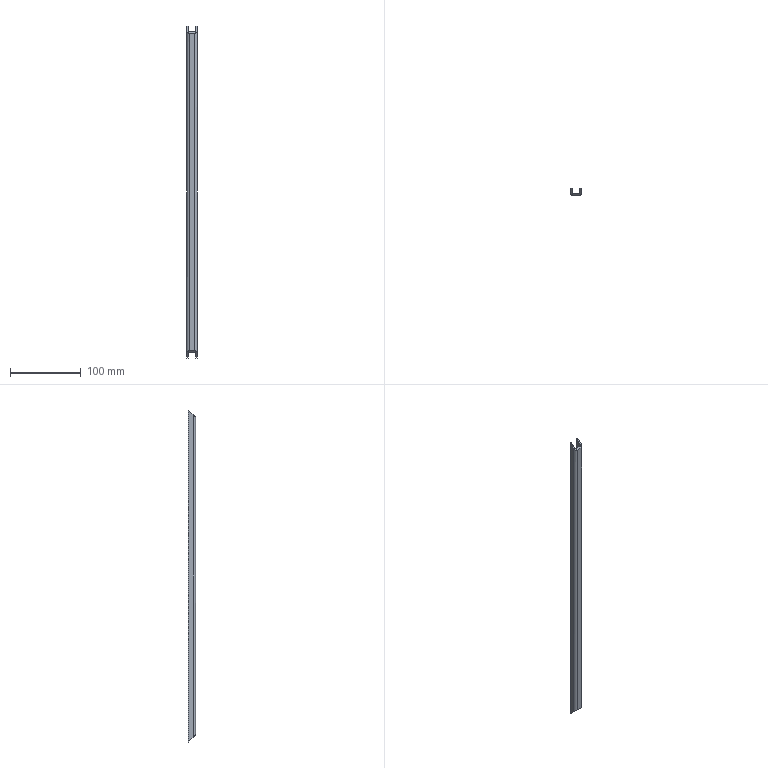Part | STEP file | 1 solid | 14 faces | box 15 x 10 x 470 mm | volume 26409 mm3 | plane 10 | cylinder 4 | commonest cylinder face diameters 3 x2 7 x2
STEP:
#1=CARTESIAN_POINT('',(0.,0.,0.));
#2=DIRECTION('',(0.,0.,1.));
#3=DIRECTION('',(1.,0.,0.));
#4=AXIS2_PLACEMENT_3D('',#1,#2,#3);
#5=CARTESIAN_POINT('',(-5.5,5.,470.));
#6=VERTEX_POINT('',#5);
#7=CARTESIAN_POINT('',(-5.5,5.,0.));
#8=VERTEX_POINT('',#7);
#9=CARTESIAN_POINT('',(-5.5,5.,470.));
#10=DIRECTION('',(0.,0.,-1.));
#11=VECTOR('',#10,1.);
#12=LINE('',#9,#11);
#13=CARTESIAN_POINT('',(-5.5,-5.,470.));
#14=DIRECTION('',(-1.,0.,0.));
#15=DIRECTION('',(0.,0.,1.));
#16=AXIS2_PLACEMENT_3D('',#13,#14,#15);
#17=PLANE('',#16);
#18=CARTESIAN_POINT('',(0.,10.));
#19=DIRECTION('',(-1.,0.));
#20=VECTOR('',#19,1.);
#21=LINE('',#18,#20);
#22=(GEOMETRIC_REPRESENTATION_CONTEXT(2)PARAMETRIC_REPRESENTATION_CONTEXT()REPRESENTATION_CONTEXT('',''));
#23=DEFINITIONAL_REPRESENTATION('',(#21),#22);
#24=PCURVE('',#17,#23);
#25=CARTESIAN_POINT('',(-7.5,5.,470.));
#26=DIRECTION('',(0.,1.,0.));
#27=DIRECTION('',(0.,0.,1.));
#28=AXIS2_PLACEMENT_3D('',#25,#26,#27);
#29=PLANE('',#28);
#30=CARTESIAN_POINT('',(0.,2.));
#31=DIRECTION('',(-1.,0.));
#32=VECTOR('',#31,1.);
#33=LINE('',#30,#32);
#34=(GEOMETRIC_REPRESENTATION_CONTEXT(2)PARAMETRIC_REPRESENTATION_CONTEXT()REPRESENTATION_CONTEXT('',''));
#35=DEFINITIONAL_REPRESENTATION('',(#33),#34);
#36=PCURVE('',#29,#35);
#37=SURFACE_CURVE('',#12,(#24,#36),.PCURVE_S1.);
#38=EDGE_CURVE('',#6,#8,#37,.T.);
#39=ORIENTED_EDGE('',*,*,#38,.F.);
#40=CARTESIAN_POINT('',(-5.5,-1.5,463.5));
#41=VERTEX_POINT('',#40);
#42=CARTESIAN_POINT('',(-5.5,0.,465.));
#43=DIRECTION('',(0.,-0.7071,-0.7071));
#44=VECTOR('',#43,1.);
#45=LINE('',#42,#44);
#46=CARTESIAN_POINT('',(-5.,5.));
#47=DIRECTION('',(-0.7071,-0.7071));
#48=VECTOR('',#47,1.);
#49=LINE('',#46,#48);
#50=(GEOMETRIC_REPRESENTATION_CONTEXT(2)PARAMETRIC_REPRESENTATION_CONTEXT()REPRESENTATION_CONTEXT('',''));
#51=DEFINITIONAL_REPRESENTATION('',(#49),#50);
#52=PCURVE('',#17,#51);
#53=CARTESIAN_POINT('',(-62.5,5.,470.));
#54=DIRECTION('',(0.,0.7071,-0.7071));
#55=DIRECTION('',(0.,0.7071,0.7071));
#56=AXIS2_PLACEMENT_3D('',#53,#54,#55);
#57=PLANE('',#56);
#58=CARTESIAN_POINT('',(-7.071,57.));
#59=DIRECTION('',(-1.,0.));
#60=VECTOR('',#59,1.);
#61=LINE('',#58,#60);
#62=(GEOMETRIC_REPRESENTATION_CONTEXT(2)PARAMETRIC_REPRESENTATION_CONTEXT()REPRESENTATION_CONTEXT('',''));
#63=DEFINITIONAL_REPRESENTATION('',(#61),#62);
#64=PCURVE('',#57,#63);
#65=SURFACE_CURVE('',#45,(#52,#64),.PCURVE_S1.);
#66=EDGE_CURVE('',#6,#41,#65,.T.);
#67=ORIENTED_EDGE('',*,*,#66,.T.);
#68=CARTESIAN_POINT('',(-5.5,-1.5,6.5));
#69=VERTEX_POINT('',#68);
#70=CARTESIAN_POINT('',(-5.5,-1.5,470.));
#71=DIRECTION('',(0.,0.,-1.));
#72=VECTOR('',#71,1.);
#73=LINE('',#70,#72);
#74=CARTESIAN_POINT('',(0.,3.5));
#75=DIRECTION('',(-1.,0.));
#76=VECTOR('',#75,1.);
#77=LINE('',#74,#76);
#78=(GEOMETRIC_REPRESENTATION_CONTEXT(2)PARAMETRIC_REPRESENTATION_CONTEXT()REPRESENTATION_CONTEXT('',''));
#79=DEFINITIONAL_REPRESENTATION('',(#77),#78);
#80=PCURVE('',#17,#79);
#81=CARTESIAN_POINT('',(-4.,-1.5,470.));
#82=DIRECTION('',(0.,0.,-1.));
#83=DIRECTION('',(-1.,0.,0.));
#84=AXIS2_PLACEMENT_3D('',#81,#82,#83);
#85=CYLINDRICAL_SURFACE('',#84,1.5);
#86=CARTESIAN_POINT('',(6.283,0.));
#87=DIRECTION('',(0.,1.));
#88=VECTOR('',#87,1.);
#89=LINE('',#86,#88);
#90=(GEOMETRIC_REPRESENTATION_CONTEXT(2)PARAMETRIC_REPRESENTATION_CONTEXT()REPRESENTATION_CONTEXT('',''));
#91=DEFINITIONAL_REPRESENTATION('',(#89),#90);
#92=PCURVE('',#85,#91);
#93=SURFACE_CURVE('',#73,(#80,#92),.PCURVE_S1.);
#94=EDGE_CURVE('',#41,#69,#93,.T.);
#95=ORIENTED_EDGE('',*,*,#94,.T.);
#96=CARTESIAN_POINT('',(-5.5,-235.,240.));
#97=DIRECTION('',(0.,0.7071,-0.7071));
#98=VECTOR('',#97,1.);
#99=LINE('',#96,#98);
#100=CARTESIAN_POINT('',(-230.,-230.));
#101=DIRECTION('',(-0.7071,0.7071));
#102=VECTOR('',#101,1.);
#103=LINE('',#100,#102);
#104=(GEOMETRIC_REPRESENTATION_CONTEXT(2)PARAMETRIC_REPRESENTATION_CONTEXT()REPRESENTATION_CONTEXT('',''));
#105=DEFINITIONAL_REPRESENTATION('',(#103),#104);
#106=PCURVE('',#17,#105);
#107=CARTESIAN_POINT('',(-62.5,5.,0.));
#108=DIRECTION('',(0.,0.7071,0.7071));
#109=DIRECTION('',(0.,-0.7071,0.7071));
#110=AXIS2_PLACEMENT_3D('',#107,#108,#109);
#111=PLANE('',#110);
#112=CARTESIAN_POINT('',(339.411,57.));
#113=DIRECTION('',(-1.,0.));
#114=VECTOR('',#113,1.);
#115=LINE('',#112,#114);
#116=(GEOMETRIC_REPRESENTATION_CONTEXT(2)PARAMETRIC_REPRESENTATION_CONTEXT()REPRESENTATION_CONTEXT('',''));
#117=DEFINITIONAL_REPRESENTATION('',(#115),#116);
#118=PCURVE('',#111,#117);
#119=SURFACE_CURVE('',#99,(#106,#118),.PCURVE_S1.);
#120=EDGE_CURVE('',#69,#8,#119,.T.);
#121=ORIENTED_EDGE('',*,*,#120,.T.);
#122=EDGE_LOOP('',(#39,#67,#95,#121));
#123=FACE_BOUND('',#122,.T.);
#124=ADVANCED_FACE('',(#123),#17,.F.);
#125=CARTESIAN_POINT('',(-7.5,5.,0.));
#126=VERTEX_POINT('',#125);
#127=CARTESIAN_POINT('',(-7.5,5.,0.));
#128=DIRECTION('',(1.,0.,0.));
#129=VECTOR('',#128,1.);
#130=LINE('',#127,#129);
#131=CARTESIAN_POINT('',(-470.,0.));
#132=DIRECTION('',(0.,1.));
#133=VECTOR('',#132,1.);
#134=LINE('',#131,#133);
#135=(GEOMETRIC_REPRESENTATION_CONTEXT(2)PARAMETRIC_REPRESENTATION_CONTEXT()REPRESENTATION_CONTEXT('',''));
#136=DEFINITIONAL_REPRESENTATION('',(#134),#135);
#137=PCURVE('',#29,#136);
#138=CARTESIAN_POINT('',(0.,55.));
#139=DIRECTION('',(0.,1.));
#140=VECTOR('',#139,1.);
#141=LINE('',#138,#140);
#142=(GEOMETRIC_REPRESENTATION_CONTEXT(2)PARAMETRIC_REPRESENTATION_CONTEXT()REPRESENTATION_CONTEXT('',''));
#143=DEFINITIONAL_REPRESENTATION('',(#141),#142);
#144=PCURVE('',#111,#143);
#145=SURFACE_CURVE('',#130,(#137,#144),.PCURVE_S1.);
#146=EDGE_CURVE('',#126,#8,#145,.T.);
#147=ORIENTED_EDGE('',*,*,#146,.F.);
#148=CARTESIAN_POINT('',(-7.5,5.,470.));
#149=VERTEX_POINT('',#148);
#150=CARTESIAN_POINT('',(-7.5,5.,470.));
#151=DIRECTION('',(0.,0.,-1.));
#152=VECTOR('',#151,1.);
#153=LINE('',#150,#152);
#154=CARTESIAN_POINT('',(0.,0.));
#155=DIRECTION('',(-1.,0.));
#156=VECTOR('',#155,1.);
#157=LINE('',#154,#156);
#158=(GEOMETRIC_REPRESENTATION_CONTEXT(2)PARAMETRIC_REPRESENTATION_CONTEXT()REPRESENTATION_CONTEXT('',''));
#159=DEFINITIONAL_REPRESENTATION('',(#157),#158);
#160=PCURVE('',#29,#159);
#161=CARTESIAN_POINT('',(-7.5,-5.,470.));
#162=DIRECTION('',(-1.,0.,0.));
#163=DIRECTION('',(0.,0.,1.));
#164=AXIS2_PLACEMENT_3D('',#161,#162,#163);
#165=PLANE('',#164);
#166=CARTESIAN_POINT('',(0.,10.));
#167=DIRECTION('',(-1.,0.));
#168=VECTOR('',#167,1.);
#169=LINE('',#166,#168);
#170=(GEOMETRIC_REPRESENTATION_CONTEXT(2)PARAMETRIC_REPRESENTATION_CONTEXT()REPRESENTATION_CONTEXT('',''));
#171=DEFINITIONAL_REPRESENTATION('',(#169),#170);
#172=PCURVE('',#165,#171);
#173=SURFACE_CURVE('',#153,(#160,#172),.PCURVE_S1.);
#174=EDGE_CURVE('',#149,#126,#173,.T.);
#175=ORIENTED_EDGE('',*,*,#174,.F.);
#176=CARTESIAN_POINT('',(-7.5,5.,470.));
#177=DIRECTION('',(1.,0.,0.));
#178=VECTOR('',#177,1.);
#179=LINE('',#176,#178);
#180=CARTESIAN_POINT('',(0.,0.));
#181=DIRECTION('',(0.,1.));
#182=VECTOR('',#181,1.);
#183=LINE('',#180,#182);
#184=(GEOMETRIC_REPRESENTATION_CONTEXT(2)PARAMETRIC_REPRESENTATION_CONTEXT()REPRESENTATION_CONTEXT('',''));
#185=DEFINITIONAL_REPRESENTATION('',(#183),#184);
#186=PCURVE('',#29,#185);
#187=CARTESIAN_POINT('',(0.,55.));
#188=DIRECTION('',(0.,1.));
#189=VECTOR('',#188,1.);
#190=LINE('',#187,#189);
#191=(GEOMETRIC_REPRESENTATION_CONTEXT(2)PARAMETRIC_REPRESENTATION_CONTEXT()REPRESENTATION_CONTEXT('',''));
#192=DEFINITIONAL_REPRESENTATION('',(#190),#191);
#193=PCURVE('',#57,#192);
#194=SURFACE_CURVE('',#179,(#186,#193),.PCURVE_S1.);
#195=EDGE_CURVE('',#149,#6,#194,.T.);
#196=ORIENTED_EDGE('',*,*,#195,.T.);
#197=ORIENTED_EDGE('',*,*,#38,.T.);
#198=EDGE_LOOP('',(#147,#175,#196,#197));
#199=FACE_BOUND('',#198,.T.);
#200=ADVANCED_FACE('',(#199),#29,.T.);
#201=CARTESIAN_POINT('',(-7.5,-1.5,463.5));
#202=VERTEX_POINT('',#201);
#203=CARTESIAN_POINT('',(-7.5,0.,465.));
#204=DIRECTION('',(0.,-0.7071,-0.7071));
#205=VECTOR('',#204,1.);
#206=LINE('',#203,#205);
#207=CARTESIAN_POINT('',(-5.,5.));
#208=DIRECTION('',(-0.7071,-0.7071));
#209=VECTOR('',#208,1.);
#210=LINE('',#207,#209);
#211=(GEOMETRIC_REPRESENTATION_CONTEXT(2)PARAMETRIC_REPRESENTATION_CONTEXT()REPRESENTATION_CONTEXT('',''));
#212=DEFINITIONAL_REPRESENTATION('',(#210),#211);
#213=PCURVE('',#165,#212);
#214=CARTESIAN_POINT('',(-7.071,55.));
#215=DIRECTION('',(-1.,0.));
#216=VECTOR('',#215,1.);
#217=LINE('',#214,#216);
#218=(GEOMETRIC_REPRESENTATION_CONTEXT(2)PARAMETRIC_REPRESENTATION_CONTEXT()REPRESENTATION_CONTEXT('',''));
#219=DEFINITIONAL_REPRESENTATION('',(#217),#218);
#220=PCURVE('',#57,#219);
#221=SURFACE_CURVE('',#206,(#213,#220),.PCURVE_S1.);
#222=EDGE_CURVE('',#149,#202,#221,.T.);
#223=ORIENTED_EDGE('',*,*,#222,.F.);
#224=ORIENTED_EDGE('',*,*,#174,.T.);
#225=CARTESIAN_POINT('',(-7.5,-1.5,6.5));
#226=VERTEX_POINT('',#225);
#227=CARTESIAN_POINT('',(-7.5,-235.,240.));
#228=DIRECTION('',(0.,0.7071,-0.7071));
#229=VECTOR('',#228,1.);
#230=LINE('',#227,#229);
#231=CARTESIAN_POINT('',(-230.,-230.));
#232=DIRECTION('',(-0.7071,0.7071));
#233=VECTOR('',#232,1.);
#234=LINE('',#231,#233);
#235=(GEOMETRIC_REPRESENTATION_CONTEXT(2)PARAMETRIC_REPRESENTATION_CONTEXT()REPRESENTATION_CONTEXT('',''));
#236=DEFINITIONAL_REPRESENTATION('',(#234),#235);
#237=PCURVE('',#165,#236);
#238=CARTESIAN_POINT('',(339.411,55.));
#239=DIRECTION('',(-1.,0.));
#240=VECTOR('',#239,1.);
#241=LINE('',#238,#240);
#242=(GEOMETRIC_REPRESENTATION_CONTEXT(2)PARAMETRIC_REPRESENTATION_CONTEXT()REPRESENTATION_CONTEXT('',''));
#243=DEFINITIONAL_REPRESENTATION('',(#241),#242);
#244=PCURVE('',#111,#243);
#245=SURFACE_CURVE('',#230,(#237,#244),.PCURVE_S1.);
#246=EDGE_CURVE('',#226,#126,#245,.T.);
#247=ORIENTED_EDGE('',*,*,#246,.F.);
#248=CARTESIAN_POINT('',(-7.5,-1.5,470.));
#249=DIRECTION('',(0.,0.,-1.));
#250=VECTOR('',#249,1.);
#251=LINE('',#248,#250);
#252=CARTESIAN_POINT('',(0.,3.5));
#253=DIRECTION('',(-1.,0.));
#254=VECTOR('',#253,1.);
#255=LINE('',#252,#254);
#256=(GEOMETRIC_REPRESENTATION_CONTEXT(2)PARAMETRIC_REPRESENTATION_CONTEXT()REPRESENTATION_CONTEXT('',''));
#257=DEFINITIONAL_REPRESENTATION('',(#255),#256);
#258=PCURVE('',#165,#257);
#259=CARTESIAN_POINT('',(-4.,-1.5,470.));
#260=DIRECTION('',(0.,0.,-1.));
#261=DIRECTION('',(-1.,0.,0.));
#262=AXIS2_PLACEMENT_3D('',#259,#260,#261);
#263=CYLINDRICAL_SURFACE('',#262,3.5);
#264=CARTESIAN_POINT('',(6.283,0.));
#265=DIRECTION('',(0.,1.));
#266=VECTOR('',#265,1.);
#267=LINE('',#264,#266);
#268=(GEOMETRIC_REPRESENTATION_CONTEXT(2)PARAMETRIC_REPRESENTATION_CONTEXT()REPRESENTATION_CONTEXT('',''));
#269=DEFINITIONAL_REPRESENTATION('',(#267),#268);
#270=PCURVE('',#263,#269);
#271=SURFACE_CURVE('',#251,(#258,#270),.PCURVE_S1.);
#272=EDGE_CURVE('',#202,#226,#271,.T.);
#273=ORIENTED_EDGE('',*,*,#272,.F.);
#274=EDGE_LOOP('',(#223,#224,#247,#273));
#275=FACE_BOUND('',#274,.T.);
#276=ADVANCED_FACE('',(#275),#165,.T.);
#277=CARTESIAN_POINT('',(-4.,-5.,460.));
#278=VERTEX_POINT('',#277);
#279=CARTESIAN_POINT('',(-7.5,-1.5,463.5));
#280=CARTESIAN_POINT('',(-7.5,-3.55,461.45));
#281=CARTESIAN_POINT('',(-6.05,-5.,460.));
#282=CARTESIAN_POINT('',(-4.,-5.,460.));
#283=(BOUNDED_CURVE()B_SPLINE_CURVE(3,(#279,#280,#281,#282),.UNSPECIFIED.,.F.,.F.)B_SPLINE_CURVE_WITH_KNOTS((4,4),(4.712,6.283),.PIECEWISE_BEZIER_KNOTS.)CURVE()GEOMETRIC_REPRESENTATION_ITEM()RATIONAL_B_SPLINE_CURVE((1.,0.8047,0.8047,1.))REPRESENTATION_ITEM(''));
#284=CARTESIAN_POINT('',(6.283,6.5));
#285=CARTESIAN_POINT('',(6.262,6.575));
#286=CARTESIAN_POINT('',(6.218,6.727));
#287=CARTESIAN_POINT('',(6.152,6.96));
#288=CARTESIAN_POINT('',(6.083,7.196));
#289=CARTESIAN_POINT('',(6.013,7.433));
#290=CARTESIAN_POINT('',(5.942,7.671));
#291=CARTESIAN_POINT('',(5.87,7.906));
#292=CARTESIAN_POINT('',(5.797,8.137));
#293=CARTESIAN_POINT('',(5.723,8.362));
#294=CARTESIAN_POINT('',(5.648,8.578));
#295=CARTESIAN_POINT('',(5.573,8.784));
#296=CARTESIAN_POINT('',(5.498,8.977));
#297=CARTESIAN_POINT('',(5.422,9.157));
#298=CARTESIAN_POINT('',(5.347,9.32));
#299=CARTESIAN_POINT('',(5.273,9.468));
#300=CARTESIAN_POINT('',(5.199,9.597));
#301=CARTESIAN_POINT('',(5.125,9.709));
#302=CARTESIAN_POINT('',(5.053,9.802));
#303=CARTESIAN_POINT('',(4.982,9.876));
#304=CARTESIAN_POINT('',(4.912,9.933));
#305=CARTESIAN_POINT('',(4.844,9.972));
#306=CARTESIAN_POINT('',(4.777,9.995));
#307=CARTESIAN_POINT('',(4.734,10.));
#308=CARTESIAN_POINT('',(4.712,10.));
#309=B_SPLINE_CURVE_WITH_KNOTS('',3,(#284,#285,#286,#287,#288,#289,#290,#291,#292,#293,#294,#295,#296,#297,#298,#299,#300,#301,#302,#303,#304,#305,#306,#307,#308),.UNSPECIFIED.,.F.,.F.,(4,1,1,1,1,1,1,1,1,1,1,1,1,1,1,1,1,1,1,1,1,1,4),(4.712,4.784,4.855,4.927,4.998,5.069,5.141,5.212,5.284,5.355,5.426,5.498,5.569,5.641,5.712,5.783,5.855,5.926,5.998,6.069,6.14,6.212,6.283),.QUASI_UNIFORM_KNOTS.);
#310=(GEOMETRIC_REPRESENTATION_CONTEXT(2)PARAMETRIC_REPRESENTATION_CONTEXT()REPRESENTATION_CONTEXT('',''));
#311=DEFINITIONAL_REPRESENTATION('',(#309),#310);
#312=PCURVE('',#263,#311);
#313=CARTESIAN_POINT('',(-9.192,55.));
#314=CARTESIAN_POINT('',(-12.092,55.));
#315=CARTESIAN_POINT('',(-14.142,56.45));
#316=CARTESIAN_POINT('',(-14.142,58.5));
#317=(BOUNDED_CURVE()B_SPLINE_CURVE(3,(#313,#314,#315,#316),.UNSPECIFIED.,.F.,.F.)B_SPLINE_CURVE_WITH_KNOTS((4,4),(4.712,6.283),.PIECEWISE_BEZIER_KNOTS.)CURVE()GEOMETRIC_REPRESENTATION_ITEM()RATIONAL_B_SPLINE_CURVE((1.,0.8047,0.8047,1.))REPRESENTATION_ITEM(''));
#318=(GEOMETRIC_REPRESENTATION_CONTEXT(2)PARAMETRIC_REPRESENTATION_CONTEXT()REPRESENTATION_CONTEXT('',''));
#319=DEFINITIONAL_REPRESENTATION('',(#317),#318);
#320=PCURVE('',#57,#319);
#321=SURFACE_CURVE('',#283,(#312,#320),.PCURVE_S1.);
#322=EDGE_CURVE('',#202,#278,#321,.T.);
#323=ORIENTED_EDGE('',*,*,#322,.F.);
#324=ORIENTED_EDGE('',*,*,#272,.T.);
#325=CARTESIAN_POINT('',(-4.,-5.,10.));
#326=VERTEX_POINT('',#325);
#327=CARTESIAN_POINT('',(-4.,-5.,10.));
#328=CARTESIAN_POINT('',(-6.05,-5.,10.));
#329=CARTESIAN_POINT('',(-7.5,-3.55,8.55));
#330=CARTESIAN_POINT('',(-7.5,-1.5,6.5));
#331=(BOUNDED_CURVE()B_SPLINE_CURVE(3,(#327,#328,#329,#330),.UNSPECIFIED.,.F.,.F.)B_SPLINE_CURVE_WITH_KNOTS((4,4),(3.142,4.712),.PIECEWISE_BEZIER_KNOTS.)CURVE()GEOMETRIC_REPRESENTATION_ITEM()RATIONAL_B_SPLINE_CURVE((1.,0.8047,0.8047,1.))REPRESENTATION_ITEM(''));
#332=CARTESIAN_POINT('',(4.712,460.));
#333=CARTESIAN_POINT('',(4.734,460.));
#334=CARTESIAN_POINT('',(4.777,460.005));
#335=CARTESIAN_POINT('',(4.844,460.028));
#336=CARTESIAN_POINT('',(4.912,460.067));
#337=CARTESIAN_POINT('',(4.982,460.124));
#338=CARTESIAN_POINT('',(5.053,460.198));
#339=CARTESIAN_POINT('',(5.125,460.291));
#340=CARTESIAN_POINT('',(5.199,460.403));
#341=CARTESIAN_POINT('',(5.273,460.532));
#342=CARTESIAN_POINT('',(5.347,460.68));
#343=CARTESIAN_POINT('',(5.422,460.843));
#344=CARTESIAN_POINT('',(5.498,461.023));
#345=CARTESIAN_POINT('',(5.573,461.216));
#346=CARTESIAN_POINT('',(5.648,461.422));
#347=CARTESIAN_POINT('',(5.723,461.638));
#348=CARTESIAN_POINT('',(5.797,461.863));
#349=CARTESIAN_POINT('',(5.87,462.094));
#350=CARTESIAN_POINT('',(5.942,462.329));
#351=CARTESIAN_POINT('',(6.013,462.567));
#352=CARTESIAN_POINT('',(6.083,462.804));
#353=CARTESIAN_POINT('',(6.152,463.04));
#354=CARTESIAN_POINT('',(6.218,463.273));
#355=CARTESIAN_POINT('',(6.262,463.425));
#356=CARTESIAN_POINT('',(6.283,463.5));
#357=B_SPLINE_CURVE_WITH_KNOTS('',3,(#332,#333,#334,#335,#336,#337,#338,#339,#340,#341,#342,#343,#344,#345,#346,#347,#348,#349,#350,#351,#352,#353,#354,#355,#356),.UNSPECIFIED.,.F.,.F.,(4,1,1,1,1,1,1,1,1,1,1,1,1,1,1,1,1,1,1,1,1,1,4),(3.142,3.213,3.284,3.356,3.427,3.499,3.57,3.641,3.713,3.784,3.856,3.927,3.998,4.07,4.141,4.213,4.284,4.355,4.427,4.498,4.57,4.641,4.712),.QUASI_UNIFORM_KNOTS.);
#358=(GEOMETRIC_REPRESENTATION_CONTEXT(2)PARAMETRIC_REPRESENTATION_CONTEXT()REPRESENTATION_CONTEXT('',''));
#359=DEFINITIONAL_REPRESENTATION('',(#357),#358);
#360=PCURVE('',#263,#359);
#361=CARTESIAN_POINT('',(14.142,58.5));
#362=CARTESIAN_POINT('',(14.142,56.45));
#363=CARTESIAN_POINT('',(12.092,55.));
#364=CARTESIAN_POINT('',(9.192,55.));
#365=(BOUNDED_CURVE()B_SPLINE_CURVE(3,(#361,#362,#363,#364),.UNSPECIFIED.,.F.,.F.)B_SPLINE_CURVE_WITH_KNOTS((4,4),(3.142,4.712),.PIECEWISE_BEZIER_KNOTS.)CURVE()GEOMETRIC_REPRESENTATION_ITEM()RATIONAL_B_SPLINE_CURVE((1.,0.8047,0.8047,1.))REPRESENTATION_ITEM(''));
#366=(GEOMETRIC_REPRESENTATION_CONTEXT(2)PARAMETRIC_REPRESENTATION_CONTEXT()REPRESENTATION_CONTEXT('',''));
#367=DEFINITIONAL_REPRESENTATION('',(#365),#366);
#368=PCURVE('',#111,#367);
#369=SURFACE_CURVE('',#331,(#360,#368),.PCURVE_S1.);
#370=EDGE_CURVE('',#326,#226,#369,.T.);
#371=ORIENTED_EDGE('',*,*,#370,.F.);
#372=CARTESIAN_POINT('',(-4.,-5.,470.));
#373=DIRECTION('',(0.,0.,-1.));
#374=VECTOR('',#373,1.);
#375=LINE('',#372,#374);
#376=CARTESIAN_POINT('',(4.712,0.));
#377=DIRECTION('',(0.,1.));
#378=VECTOR('',#377,1.);
#379=LINE('',#376,#378);
#380=(GEOMETRIC_REPRESENTATION_CONTEXT(2)PARAMETRIC_REPRESENTATION_CONTEXT()REPRESENTATION_CONTEXT('',''));
#381=DEFINITIONAL_REPRESENTATION('',(#379),#380);
#382=PCURVE('',#263,#381);
#383=CARTESIAN_POINT('',(-7.5,-5.,470.));
#384=DIRECTION('',(0.,-1.,0.));
#385=DIRECTION('',(0.,0.,-1.));
#386=AXIS2_PLACEMENT_3D('',#383,#384,#385);
#387=PLANE('',#386);
#388=CARTESIAN_POINT('',(0.,3.5));
#389=DIRECTION('',(1.,0.));
#390=VECTOR('',#389,1.);
#391=LINE('',#388,#390);
#392=(GEOMETRIC_REPRESENTATION_CONTEXT(2)PARAMETRIC_REPRESENTATION_CONTEXT()REPRESENTATION_CONTEXT('',''));
#393=DEFINITIONAL_REPRESENTATION('',(#391),#392);
#394=PCURVE('',#387,#393);
#395=SURFACE_CURVE('',#375,(#382,#394),.PCURVE_S1.);
#396=EDGE_CURVE('',#278,#326,#395,.T.);
#397=ORIENTED_EDGE('',*,*,#396,.F.);
#398=EDGE_LOOP('',(#323,#324,#371,#397));
#399=FACE_BOUND('',#398,.T.);
#400=ADVANCED_FACE('',(#399),#263,.T.);
#401=CARTESIAN_POINT('',(4.,-5.,460.));
#402=VERTEX_POINT('',#401);
#403=CARTESIAN_POINT('',(-62.5,-5.,460.));
#404=DIRECTION('',(1.,0.,0.));
#405=VECTOR('',#404,1.);
#406=LINE('',#403,#405);
#407=CARTESIAN_POINT('',(10.,-55.));
#408=DIRECTION('',(0.,1.));
#409=VECTOR('',#408,1.);
#410=LINE('',#407,#409);
#411=(GEOMETRIC_REPRESENTATION_CONTEXT(2)PARAMETRIC_REPRESENTATION_CONTEXT()REPRESENTATION_CONTEXT('',''));
#412=DEFINITIONAL_REPRESENTATION('',(#410),#411);
#413=PCURVE('',#387,#412);
#414=CARTESIAN_POINT('',(-14.142,0.));
#415=DIRECTION('',(0.,1.));
#416=VECTOR('',#415,1.);
#417=LINE('',#414,#416);
#418=(GEOMETRIC_REPRESENTATION_CONTEXT(2)PARAMETRIC_REPRESENTATION_CONTEXT()REPRESENTATION_CONTEXT('',''));
#419=DEFINITIONAL_REPRESENTATION('',(#417),#418);
#420=PCURVE('',#57,#419);
#421=SURFACE_CURVE('',#406,(#413,#420),.PCURVE_S1.);
#422=EDGE_CURVE('',#278,#402,#421,.T.);
#423=ORIENTED_EDGE('',*,*,#422,.F.);
#424=ORIENTED_EDGE('',*,*,#396,.T.);
#425=CARTESIAN_POINT('',(4.,-5.,10.));
#426=VERTEX_POINT('',#425);
#427=CARTESIAN_POINT('',(-62.5,-5.,10.));
#428=DIRECTION('',(1.,0.,0.));
#429=VECTOR('',#428,1.);
#430=LINE('',#427,#429);
#431=CARTESIAN_POINT('',(460.,-55.));
#432=DIRECTION('',(0.,1.));
#433=VECTOR('',#432,1.);
#434=LINE('',#431,#433);
#435=(GEOMETRIC_REPRESENTATION_CONTEXT(2)PARAMETRIC_REPRESENTATION_CONTEXT()REPRESENTATION_CONTEXT('',''));
#436=DEFINITIONAL_REPRESENTATION('',(#434),#435);
#437=PCURVE('',#387,#436);
#438=CARTESIAN_POINT('',(14.142,0.));
#439=DIRECTION('',(0.,1.));
#440=VECTOR('',#439,1.);
#441=LINE('',#438,#440);
#442=(GEOMETRIC_REPRESENTATION_CONTEXT(2)PARAMETRIC_REPRESENTATION_CONTEXT()REPRESENTATION_CONTEXT('',''));
#443=DEFINITIONAL_REPRESENTATION('',(#441),#442);
#444=PCURVE('',#111,#443);
#445=SURFACE_CURVE('',#430,(#437,#444),.PCURVE_S1.);
#446=EDGE_CURVE('',#326,#426,#445,.T.);
#447=ORIENTED_EDGE('',*,*,#446,.T.);
#448=CARTESIAN_POINT('',(4.,-5.,470.));
#449=DIRECTION('',(0.,0.,-1.));
#450=VECTOR('',#449,1.);
#451=LINE('',#448,#450);
#452=CARTESIAN_POINT('',(0.,11.5));
#453=DIRECTION('',(1.,0.));
#454=VECTOR('',#453,1.);
#455=LINE('',#452,#454);
#456=(GEOMETRIC_REPRESENTATION_CONTEXT(2)PARAMETRIC_REPRESENTATION_CONTEXT()REPRESENTATION_CONTEXT('',''));
#457=DEFINITIONAL_REPRESENTATION('',(#455),#456);
#458=PCURVE('',#387,#457);
#459=CARTESIAN_POINT('',(4.,-1.5,470.));
#460=DIRECTION('',(0.,0.,-1.));
#461=DIRECTION('',(-1.,0.,0.));
#462=AXIS2_PLACEMENT_3D('',#459,#460,#461);
#463=CYLINDRICAL_SURFACE('',#462,3.5);
#464=CARTESIAN_POINT('',(4.712,0.));
#465=DIRECTION('',(0.,1.));
#466=VECTOR('',#465,1.);
#467=LINE('',#464,#466);
#468=(GEOMETRIC_REPRESENTATION_CONTEXT(2)PARAMETRIC_REPRESENTATION_CONTEXT()REPRESENTATION_CONTEXT('',''));
#469=DEFINITIONAL_REPRESENTATION('',(#467),#468);
#470=PCURVE('',#463,#469);
#471=SURFACE_CURVE('',#451,(#458,#470),.PCURVE_S1.);
#472=EDGE_CURVE('',#402,#426,#471,.T.);
#473=ORIENTED_EDGE('',*,*,#472,.F.);
#474=EDGE_LOOP('',(#423,#424,#447,#473));
#475=FACE_BOUND('',#474,.T.);
#476=ADVANCED_FACE('',(#475),#387,.T.);
#477=CARTESIAN_POINT('',(7.5,-1.5,463.5));
#478=VERTEX_POINT('',#477);
#479=CARTESIAN_POINT('',(4.,-5.,460.));
#480=CARTESIAN_POINT('',(6.05,-5.,460.));
#481=CARTESIAN_POINT('',(7.5,-3.55,461.45));
#482=CARTESIAN_POINT('',(7.5,-1.5,463.5));
#483=(BOUNDED_CURVE()B_SPLINE_CURVE(3,(#479,#480,#481,#482),.UNSPECIFIED.,.F.,.F.)B_SPLINE_CURVE_WITH_KNOTS((4,4),(0.,1.571),.PIECEWISE_BEZIER_KNOTS.)CURVE()GEOMETRIC_REPRESENTATION_ITEM()RATIONAL_B_SPLINE_CURVE((1.,0.8047,0.8047,1.))REPRESENTATION_ITEM(''));
#484=CARTESIAN_POINT('',(4.712,10.));
#485=CARTESIAN_POINT('',(4.691,10.));
#486=CARTESIAN_POINT('',(4.648,9.995));
#487=CARTESIAN_POINT('',(4.581,9.972));
#488=CARTESIAN_POINT('',(4.512,9.933));
#489=CARTESIAN_POINT('',(4.443,9.876));
#490=CARTESIAN_POINT('',(4.372,9.802));
#491=CARTESIAN_POINT('',(4.299,9.709));
#492=CARTESIAN_POINT('',(4.226,9.597));
#493=CARTESIAN_POINT('',(4.152,9.468));
#494=CARTESIAN_POINT('',(4.077,9.32));
#495=CARTESIAN_POINT('',(4.002,9.157));
#496=CARTESIAN_POINT('',(3.927,8.977));
#497=CARTESIAN_POINT('',(3.852,8.784));
#498=CARTESIAN_POINT('',(3.777,8.578));
#499=CARTESIAN_POINT('',(3.702,8.362));
#500=CARTESIAN_POINT('',(3.628,8.137));
#501=CARTESIAN_POINT('',(3.555,7.906));
#502=CARTESIAN_POINT('',(3.482,7.671));
#503=CARTESIAN_POINT('',(3.411,7.433));
#504=CARTESIAN_POINT('',(3.342,7.196));
#505=CARTESIAN_POINT('',(3.273,6.96));
#506=CARTESIAN_POINT('',(3.206,6.727));
#507=CARTESIAN_POINT('',(3.163,6.575));
#508=CARTESIAN_POINT('',(3.142,6.5));
#509=B_SPLINE_CURVE_WITH_KNOTS('',3,(#484,#485,#486,#487,#488,#489,#490,#491,#492,#493,#494,#495,#496,#497,#498,#499,#500,#501,#502,#503,#504,#505,#506,#507,#508),.UNSPECIFIED.,.F.,.F.,(4,1,1,1,1,1,1,1,1,1,1,1,1,1,1,1,1,1,1,1,1,1,4),(0.,0.0714,0.1428,0.2142,0.2856,0.357,0.4284,0.4998,0.5712,0.6426,0.714,0.7854,0.8568,0.9282,0.9996,1.071,1.142,1.214,1.285,1.357,1.428,1.499,1.571),.QUASI_UNIFORM_KNOTS.);
#510=(GEOMETRIC_REPRESENTATION_CONTEXT(2)PARAMETRIC_REPRESENTATION_CONTEXT()REPRESENTATION_CONTEXT('',''));
#511=DEFINITIONAL_REPRESENTATION('',(#509),#510);
#512=PCURVE('',#463,#511);
#513=CARTESIAN_POINT('',(-14.142,66.5));
#514=CARTESIAN_POINT('',(-14.142,68.55));
#515=CARTESIAN_POINT('',(-12.092,70.));
#516=CARTESIAN_POINT('',(-9.192,70.));
#517=(BOUNDED_CURVE()B_SPLINE_CURVE(3,(#513,#514,#515,#516),.UNSPECIFIED.,.F.,.F.)B_SPLINE_CURVE_WITH_KNOTS((4,4),(0.,1.571),.PIECEWISE_BEZIER_KNOTS.)CURVE()GEOMETRIC_REPRESENTATION_ITEM()RATIONAL_B_SPLINE_CURVE((1.,0.8047,0.8047,1.))REPRESENTATION_ITEM(''));
#518=(GEOMETRIC_REPRESENTATION_CONTEXT(2)PARAMETRIC_REPRESENTATION_CONTEXT()REPRESENTATION_CONTEXT('',''));
#519=DEFINITIONAL_REPRESENTATION('',(#517),#518);
#520=PCURVE('',#57,#519);
#521=SURFACE_CURVE('',#483,(#512,#520),.PCURVE_S1.);
#522=EDGE_CURVE('',#402,#478,#521,.T.);
#523=ORIENTED_EDGE('',*,*,#522,.F.);
#524=ORIENTED_EDGE('',*,*,#472,.T.);
#525=CARTESIAN_POINT('',(7.5,-1.5,6.5));
#526=VERTEX_POINT('',#525);
#527=CARTESIAN_POINT('',(7.5,-1.5,6.5));
#528=CARTESIAN_POINT('',(7.5,-3.55,8.55));
#529=CARTESIAN_POINT('',(6.05,-5.,10.));
#530=CARTESIAN_POINT('',(4.,-5.,10.));
#531=(BOUNDED_CURVE()B_SPLINE_CURVE(3,(#527,#528,#529,#530),.UNSPECIFIED.,.F.,.F.)B_SPLINE_CURVE_WITH_KNOTS((4,4),(1.571,3.142),.PIECEWISE_BEZIER_KNOTS.)CURVE()GEOMETRIC_REPRESENTATION_ITEM()RATIONAL_B_SPLINE_CURVE((1.,0.8047,0.8047,1.))REPRESENTATION_ITEM(''));
#532=CARTESIAN_POINT('',(3.142,463.5));
#533=CARTESIAN_POINT('',(3.163,463.425));
#534=CARTESIAN_POINT('',(3.206,463.273));
#535=CARTESIAN_POINT('',(3.273,463.04));
#536=CARTESIAN_POINT('',(3.342,462.804));
#537=CARTESIAN_POINT('',(3.411,462.567));
#538=CARTESIAN_POINT('',(3.482,462.329));
#539=CARTESIAN_POINT('',(3.555,462.094));
#540=CARTESIAN_POINT('',(3.628,461.863));
#541=CARTESIAN_POINT('',(3.702,461.638));
#542=CARTESIAN_POINT('',(3.777,461.422));
#543=CARTESIAN_POINT('',(3.852,461.216));
#544=CARTESIAN_POINT('',(3.927,461.023));
#545=CARTESIAN_POINT('',(4.002,460.843));
#546=CARTESIAN_POINT('',(4.077,460.68));
#547=CARTESIAN_POINT('',(4.152,460.532));
#548=CARTESIAN_POINT('',(4.226,460.403));
#549=CARTESIAN_POINT('',(4.299,460.291));
#550=CARTESIAN_POINT('',(4.372,460.198));
#551=CARTESIAN_POINT('',(4.443,460.124));
#552=CARTESIAN_POINT('',(4.512,460.067));
#553=CARTESIAN_POINT('',(4.581,460.028));
#554=CARTESIAN_POINT('',(4.648,460.005));
#555=CARTESIAN_POINT('',(4.691,460.));
#556=CARTESIAN_POINT('',(4.712,460.));
#557=B_SPLINE_CURVE_WITH_KNOTS('',3,(#532,#533,#534,#535,#536,#537,#538,#539,#540,#541,#542,#543,#544,#545,#546,#547,#548,#549,#550,#551,#552,#553,#554,#555,#556),.UNSPECIFIED.,.F.,.F.,(4,1,1,1,1,1,1,1,1,1,1,1,1,1,1,1,1,1,1,1,1,1,4),(1.571,1.642,1.714,1.785,1.856,1.928,1.999,2.071,2.142,2.213,2.285,2.356,2.428,2.499,2.57,2.642,2.713,2.785,2.856,2.927,2.999,3.07,3.142),.QUASI_UNIFORM_KNOTS.);
#558=(GEOMETRIC_REPRESENTATION_CONTEXT(2)PARAMETRIC_REPRESENTATION_CONTEXT()REPRESENTATION_CONTEXT('',''));
#559=DEFINITIONAL_REPRESENTATION('',(#557),#558);
#560=PCURVE('',#463,#559);
#561=CARTESIAN_POINT('',(9.192,70.));
#562=CARTESIAN_POINT('',(12.092,70.));
#563=CARTESIAN_POINT('',(14.142,68.55));
#564=CARTESIAN_POINT('',(14.142,66.5));
#565=(BOUNDED_CURVE()B_SPLINE_CURVE(3,(#561,#562,#563,#564),.UNSPECIFIED.,.F.,.F.)B_SPLINE_CURVE_WITH_KNOTS((4,4),(1.571,3.142),.PIECEWISE_BEZIER_KNOTS.)CURVE()GEOMETRIC_REPRESENTATION_ITEM()RATIONAL_B_SPLINE_CURVE((1.,0.8047,0.8047,1.))REPRESENTATION_ITEM(''));
#566=(GEOMETRIC_REPRESENTATION_CONTEXT(2)PARAMETRIC_REPRESENTATION_CONTEXT()REPRESENTATION_CONTEXT('',''));
#567=DEFINITIONAL_REPRESENTATION('',(#565),#566);
#568=PCURVE('',#111,#567);
#569=SURFACE_CURVE('',#531,(#560,#568),.PCURVE_S1.);
#570=EDGE_CURVE('',#526,#426,#569,.T.);
#571=ORIENTED_EDGE('',*,*,#570,.F.);
#572=CARTESIAN_POINT('',(7.5,-1.5,470.));
#573=DIRECTION('',(0.,0.,-1.));
#574=VECTOR('',#573,1.);
#575=LINE('',#572,#574);
#576=CARTESIAN_POINT('',(3.142,0.));
#577=DIRECTION('',(0.,1.));
#578=VECTOR('',#577,1.);
#579=LINE('',#576,#578);
#580=(GEOMETRIC_REPRESENTATION_CONTEXT(2)PARAMETRIC_REPRESENTATION_CONTEXT()REPRESENTATION_CONTEXT('',''));
#581=DEFINITIONAL_REPRESENTATION('',(#579),#580);
#582=PCURVE('',#463,#581);
#583=CARTESIAN_POINT('',(7.5,-5.,470.));
#584=DIRECTION('',(1.,0.,0.));
#585=DIRECTION('',(0.,0.,-1.));
#586=AXIS2_PLACEMENT_3D('',#583,#584,#585);
#587=PLANE('',#586);
#588=CARTESIAN_POINT('',(0.,3.5));
#589=DIRECTION('',(1.,0.));
#590=VECTOR('',#589,1.);
#591=LINE('',#588,#590);
#592=(GEOMETRIC_REPRESENTATION_CONTEXT(2)PARAMETRIC_REPRESENTATION_CONTEXT()REPRESENTATION_CONTEXT('',''));
#593=DEFINITIONAL_REPRESENTATION('',(#591),#592);
#594=PCURVE('',#587,#593);
#595=SURFACE_CURVE('',#575,(#582,#594),.PCURVE_S1.);
#596=EDGE_CURVE('',#478,#526,#595,.T.);
#597=ORIENTED_EDGE('',*,*,#596,.F.);
#598=EDGE_LOOP('',(#523,#524,#571,#597));
#599=FACE_BOUND('',#598,.T.);
#600=ADVANCED_FACE('',(#599),#463,.T.);
#601=CARTESIAN_POINT('',(7.5,5.,470.));
#602=VERTEX_POINT('',#601);
#603=CARTESIAN_POINT('',(7.5,5.,470.));
#604=DIRECTION('',(0.,0.7071,0.7071));
#605=VECTOR('',#604,1.);
#606=LINE('',#603,#605);
#607=CARTESIAN_POINT('',(0.,10.));
#608=DIRECTION('',(-0.7071,0.7071));
#609=VECTOR('',#608,1.);
#610=LINE('',#607,#609);
#611=(GEOMETRIC_REPRESENTATION_CONTEXT(2)PARAMETRIC_REPRESENTATION_CONTEXT()REPRESENTATION_CONTEXT('',''));
#612=DEFINITIONAL_REPRESENTATION('',(#610),#611);
#613=PCURVE('',#587,#612);
#614=CARTESIAN_POINT('',(0.,70.));
#615=DIRECTION('',(1.,0.));
#616=VECTOR('',#615,1.);
#617=LINE('',#614,#616);
#618=(GEOMETRIC_REPRESENTATION_CONTEXT(2)PARAMETRIC_REPRESENTATION_CONTEXT()REPRESENTATION_CONTEXT('',''));
#619=DEFINITIONAL_REPRESENTATION('',(#617),#618);
#620=PCURVE('',#57,#619);
#621=SURFACE_CURVE('',#606,(#613,#620),.PCURVE_S1.);
#622=EDGE_CURVE('',#478,#602,#621,.T.);
#623=ORIENTED_EDGE('',*,*,#622,.F.);
#624=ORIENTED_EDGE('',*,*,#596,.T.);
#625=CARTESIAN_POINT('',(7.5,5.,0.));
#626=VERTEX_POINT('',#625);
#627=CARTESIAN_POINT('',(7.5,5.,0.));
#628=DIRECTION('',(0.,-0.7071,0.7071));
#629=VECTOR('',#628,1.);
#630=LINE('',#627,#629);
#631=CARTESIAN_POINT('',(470.,10.));
#632=DIRECTION('',(-0.7071,-0.7071));
#633=VECTOR('',#632,1.);
#634=LINE('',#631,#633);
#635=(GEOMETRIC_REPRESENTATION_CONTEXT(2)PARAMETRIC_REPRESENTATION_CONTEXT()REPRESENTATION_CONTEXT('',''));
#636=DEFINITIONAL_REPRESENTATION('',(#634),#635);
#637=PCURVE('',#587,#636);
#638=CARTESIAN_POINT('',(0.,70.));
#639=DIRECTION('',(1.,0.));
#640=VECTOR('',#639,1.);
#641=LINE('',#638,#640);
#642=(GEOMETRIC_REPRESENTATION_CONTEXT(2)PARAMETRIC_REPRESENTATION_CONTEXT()REPRESENTATION_CONTEXT('',''));
#643=DEFINITIONAL_REPRESENTATION('',(#641),#642);
#644=PCURVE('',#111,#643);
#645=SURFACE_CURVE('',#630,(#637,#644),.PCURVE_S1.);
#646=EDGE_CURVE('',#626,#526,#645,.T.);
#647=ORIENTED_EDGE('',*,*,#646,.F.);
#648=CARTESIAN_POINT('',(7.5,5.,470.));
#649=DIRECTION('',(0.,0.,-1.));
#650=VECTOR('',#649,1.);
#651=LINE('',#648,#650);
#652=CARTESIAN_POINT('',(0.,10.));
#653=DIRECTION('',(1.,0.));
#654=VECTOR('',#653,1.);
#655=LINE('',#652,#654);
#656=(GEOMETRIC_REPRESENTATION_CONTEXT(2)PARAMETRIC_REPRESENTATION_CONTEXT()REPRESENTATION_CONTEXT('',''));
#657=DEFINITIONAL_REPRESENTATION('',(#655),#656);
#658=PCURVE('',#587,#657);
#659=CARTESIAN_POINT('',(5.5,5.,470.));
#660=DIRECTION('',(0.,1.,0.));
#661=DIRECTION('',(0.,0.,1.));
#662=AXIS2_PLACEMENT_3D('',#659,#660,#661);
#663=PLANE('',#662);
#664=CARTESIAN_POINT('',(0.,2.));
#665=DIRECTION('',(-1.,0.));
#666=VECTOR('',#665,1.);
#667=LINE('',#664,#666);
#668=(GEOMETRIC_REPRESENTATION_CONTEXT(2)PARAMETRIC_REPRESENTATION_CONTEXT()REPRESENTATION_CONTEXT('',''));
#669=DEFINITIONAL_REPRESENTATION('',(#667),#668);
#670=PCURVE('',#663,#669);
#671=SURFACE_CURVE('',#651,(#658,#670),.PCURVE_S1.);
#672=EDGE_CURVE('',#602,#626,#671,.T.);
#673=ORIENTED_EDGE('',*,*,#672,.F.);
#674=EDGE_LOOP('',(#623,#624,#647,#673));
#675=FACE_BOUND('',#674,.T.);
#676=ADVANCED_FACE('',(#675),#587,.T.);
#677=CARTESIAN_POINT('',(5.5,5.,0.));
#678=VERTEX_POINT('',#677);
#679=CARTESIAN_POINT('',(5.5,5.,0.));
#680=DIRECTION('',(1.,0.,0.));
#681=VECTOR('',#680,1.);
#682=LINE('',#679,#681);
#683=CARTESIAN_POINT('',(-470.,0.));
#684=DIRECTION('',(0.,1.));
#685=VECTOR('',#684,1.);
#686=LINE('',#683,#685);
#687=(GEOMETRIC_REPRESENTATION_CONTEXT(2)PARAMETRIC_REPRESENTATION_CONTEXT()REPRESENTATION_CONTEXT('',''));
#688=DEFINITIONAL_REPRESENTATION('',(#686),#687);
#689=PCURVE('',#663,#688);
#690=CARTESIAN_POINT('',(0.,68.));
#691=DIRECTION('',(0.,1.));
#692=VECTOR('',#691,1.);
#693=LINE('',#690,#692);
#694=(GEOMETRIC_REPRESENTATION_CONTEXT(2)PARAMETRIC_REPRESENTATION_CONTEXT()REPRESENTATION_CONTEXT('',''));
#695=DEFINITIONAL_REPRESENTATION('',(#693),#694);
#696=PCURVE('',#111,#695);
#697=SURFACE_CURVE('',#682,(#689,#696),.PCURVE_S1.);
#698=EDGE_CURVE('',#678,#626,#697,.T.);
#699=ORIENTED_EDGE('',*,*,#698,.F.);
#700=CARTESIAN_POINT('',(5.5,5.,470.));
#701=VERTEX_POINT('',#700);
#702=CARTESIAN_POINT('',(5.5,5.,470.));
#703=DIRECTION('',(0.,0.,-1.));
#704=VECTOR('',#703,1.);
#705=LINE('',#702,#704);
#706=CARTESIAN_POINT('',(0.,0.));
#707=DIRECTION('',(-1.,0.));
#708=VECTOR('',#707,1.);
#709=LINE('',#706,#708);
#710=(GEOMETRIC_REPRESENTATION_CONTEXT(2)PARAMETRIC_REPRESENTATION_CONTEXT()REPRESENTATION_CONTEXT('',''));
#711=DEFINITIONAL_REPRESENTATION('',(#709),#710);
#712=PCURVE('',#663,#711);
#713=CARTESIAN_POINT('',(5.5,-5.,470.));
#714=DIRECTION('',(1.,0.,0.));
#715=DIRECTION('',(0.,0.,-1.));
#716=AXIS2_PLACEMENT_3D('',#713,#714,#715);
#717=PLANE('',#716);
#718=CARTESIAN_POINT('',(0.,10.));
#719=DIRECTION('',(1.,0.));
#720=VECTOR('',#719,1.);
#721=LINE('',#718,#720);
#722=(GEOMETRIC_REPRESENTATION_CONTEXT(2)PARAMETRIC_REPRESENTATION_CONTEXT()REPRESENTATION_CONTEXT('',''));
#723=DEFINITIONAL_REPRESENTATION('',(#721),#722);
#724=PCURVE('',#717,#723);
#725=SURFACE_CURVE('',#705,(#712,#724),.PCURVE_S1.);
#726=EDGE_CURVE('',#701,#678,#725,.T.);
#727=ORIENTED_EDGE('',*,*,#726,.F.);
#728=CARTESIAN_POINT('',(5.5,5.,470.));
#729=DIRECTION('',(1.,0.,0.));
#730=VECTOR('',#729,1.);
#731=LINE('',#728,#730);
#732=CARTESIAN_POINT('',(0.,0.));
#733=DIRECTION('',(0.,1.));
#734=VECTOR('',#733,1.);
#735=LINE('',#732,#734);
#736=(GEOMETRIC_REPRESENTATION_CONTEXT(2)PARAMETRIC_REPRESENTATION_CONTEXT()REPRESENTATION_CONTEXT('',''));
#737=DEFINITIONAL_REPRESENTATION('',(#735),#736);
#738=PCURVE('',#663,#737);
#739=CARTESIAN_POINT('',(0.,68.));
#740=DIRECTION('',(0.,1.));
#741=VECTOR('',#740,1.);
#742=LINE('',#739,#741);
#743=(GEOMETRIC_REPRESENTATION_CONTEXT(2)PARAMETRIC_REPRESENTATION_CONTEXT()REPRESENTATION_CONTEXT('',''));
#744=DEFINITIONAL_REPRESENTATION('',(#742),#743);
#745=PCURVE('',#57,#744);
#746=SURFACE_CURVE('',#731,(#738,#745),.PCURVE_S1.);
#747=EDGE_CURVE('',#701,#602,#746,.T.);
#748=ORIENTED_EDGE('',*,*,#747,.T.);
#749=ORIENTED_EDGE('',*,*,#672,.T.);
#750=EDGE_LOOP('',(#699,#727,#748,#749));
#751=FACE_BOUND('',#750,.T.);
#752=ADVANCED_FACE('',(#751),#663,.T.);
#753=CARTESIAN_POINT('',(5.5,-1.5,463.5));
#754=VERTEX_POINT('',#753);
#755=CARTESIAN_POINT('',(5.5,-1.5,6.5));
#756=VERTEX_POINT('',#755);
#757=CARTESIAN_POINT('',(5.5,-1.5,470.));
#758=DIRECTION('',(0.,0.,-1.));
#759=VECTOR('',#758,1.);
#760=LINE('',#757,#759);
#761=CARTESIAN_POINT('',(0.,3.5));
#762=DIRECTION('',(1.,0.));
#763=VECTOR('',#762,1.);
#764=LINE('',#761,#763);
#765=(GEOMETRIC_REPRESENTATION_CONTEXT(2)PARAMETRIC_REPRESENTATION_CONTEXT()REPRESENTATION_CONTEXT('',''));
#766=DEFINITIONAL_REPRESENTATION('',(#764),#765);
#767=PCURVE('',#717,#766);
#768=CARTESIAN_POINT('',(4.,-1.5,470.));
#769=DIRECTION('',(0.,0.,-1.));
#770=DIRECTION('',(-1.,0.,0.));
#771=AXIS2_PLACEMENT_3D('',#768,#769,#770);
#772=CYLINDRICAL_SURFACE('',#771,1.5);
#773=CARTESIAN_POINT('',(3.142,0.));
#774=DIRECTION('',(0.,1.));
#775=VECTOR('',#774,1.);
#776=LINE('',#773,#775);
#777=(GEOMETRIC_REPRESENTATION_CONTEXT(2)PARAMETRIC_REPRESENTATION_CONTEXT()REPRESENTATION_CONTEXT('',''));
#778=DEFINITIONAL_REPRESENTATION('',(#776),#777);
#779=PCURVE('',#772,#778);
#780=SURFACE_CURVE('',#760,(#767,#779),.PCURVE_S1.);
#781=EDGE_CURVE('',#754,#756,#780,.T.);
#782=ORIENTED_EDGE('',*,*,#781,.F.);
#783=CARTESIAN_POINT('',(5.5,0.,465.));
#784=DIRECTION('',(0.,0.7071,0.7071));
#785=VECTOR('',#784,1.);
#786=LINE('',#783,#785);
#787=CARTESIAN_POINT('',(5.,5.));
#788=DIRECTION('',(-0.7071,0.7071));
#789=VECTOR('',#788,1.);
#790=LINE('',#787,#789);
#791=(GEOMETRIC_REPRESENTATION_CONTEXT(2)PARAMETRIC_REPRESENTATION_CONTEXT()REPRESENTATION_CONTEXT('',''));
#792=DEFINITIONAL_REPRESENTATION('',(#790),#791);
#793=PCURVE('',#717,#792);
#794=CARTESIAN_POINT('',(-7.071,68.));
#795=DIRECTION('',(1.,0.));
#796=VECTOR('',#795,1.);
#797=LINE('',#794,#796);
#798=(GEOMETRIC_REPRESENTATION_CONTEXT(2)PARAMETRIC_REPRESENTATION_CONTEXT()REPRESENTATION_CONTEXT('',''));
#799=DEFINITIONAL_REPRESENTATION('',(#797),#798);
#800=PCURVE('',#57,#799);
#801=SURFACE_CURVE('',#786,(#793,#800),.PCURVE_S1.);
#802=EDGE_CURVE('',#754,#701,#801,.T.);
#803=ORIENTED_EDGE('',*,*,#802,.T.);
#804=ORIENTED_EDGE('',*,*,#726,.T.);
#805=CARTESIAN_POINT('',(5.5,-235.,240.));
#806=DIRECTION('',(0.,-0.7071,0.7071));
#807=VECTOR('',#806,1.);
#808=LINE('',#805,#807);
#809=CARTESIAN_POINT('',(230.,-230.));
#810=DIRECTION('',(-0.7071,-0.7071));
#811=VECTOR('',#810,1.);
#812=LINE('',#809,#811);
#813=(GEOMETRIC_REPRESENTATION_CONTEXT(2)PARAMETRIC_REPRESENTATION_CONTEXT()REPRESENTATION_CONTEXT('',''));
#814=DEFINITIONAL_REPRESENTATION('',(#812),#813);
#815=PCURVE('',#717,#814);
#816=CARTESIAN_POINT('',(339.411,68.));
#817=DIRECTION('',(1.,0.));
#818=VECTOR('',#817,1.);
#819=LINE('',#816,#818);
#820=(GEOMETRIC_REPRESENTATION_CONTEXT(2)PARAMETRIC_REPRESENTATION_CONTEXT()REPRESENTATION_CONTEXT('',''));
#821=DEFINITIONAL_REPRESENTATION('',(#819),#820);
#822=PCURVE('',#111,#821);
#823=SURFACE_CURVE('',#808,(#815,#822),.PCURVE_S1.);
#824=EDGE_CURVE('',#678,#756,#823,.T.);
#825=ORIENTED_EDGE('',*,*,#824,.T.);
#826=EDGE_LOOP('',(#782,#803,#804,#825));
#827=FACE_BOUND('',#826,.T.);
#828=ADVANCED_FACE('',(#827),#717,.F.);
#829=CARTESIAN_POINT('',(4.,-3.,8.));
#830=VERTEX_POINT('',#829);
#831=CARTESIAN_POINT('',(5.5,-1.5,6.5));
#832=CARTESIAN_POINT('',(5.5,-2.379,7.379));
#833=CARTESIAN_POINT('',(4.879,-3.,8.));
#834=CARTESIAN_POINT('',(4.,-3.,8.));
#835=(BOUNDED_CURVE()B_SPLINE_CURVE(3,(#831,#832,#833,#834),.UNSPECIFIED.,.F.,.F.)B_SPLINE_CURVE_WITH_KNOTS((4,4),(1.571,3.142),.PIECEWISE_BEZIER_KNOTS.)CURVE()GEOMETRIC_REPRESENTATION_ITEM()RATIONAL_B_SPLINE_CURVE((1.,0.8047,0.8047,1.))REPRESENTATION_ITEM(''));
#836=CARTESIAN_POINT('',(3.142,463.5));
#837=CARTESIAN_POINT('',(3.163,463.468));
#838=CARTESIAN_POINT('',(3.206,463.403));
#839=CARTESIAN_POINT('',(3.273,463.303));
#840=CARTESIAN_POINT('',(3.342,463.202));
#841=CARTESIAN_POINT('',(3.411,463.1));
#842=CARTESIAN_POINT('',(3.482,462.998));
#843=CARTESIAN_POINT('',(3.555,462.897));
#844=CARTESIAN_POINT('',(3.628,462.798));
#845=CARTESIAN_POINT('',(3.702,462.702));
#846=CARTESIAN_POINT('',(3.777,462.609));
#847=CARTESIAN_POINT('',(3.852,462.521));
#848=CARTESIAN_POINT('',(3.927,462.438));
#849=CARTESIAN_POINT('',(4.002,462.361));
#850=CARTESIAN_POINT('',(4.077,462.291));
#851=CARTESIAN_POINT('',(4.152,462.228));
#852=CARTESIAN_POINT('',(4.226,462.173));
#853=CARTESIAN_POINT('',(4.299,462.125));
#854=CARTESIAN_POINT('',(4.372,462.085));
#855=CARTESIAN_POINT('',(4.443,462.053));
#856=CARTESIAN_POINT('',(4.512,462.029));
#857=CARTESIAN_POINT('',(4.581,462.012));
#858=CARTESIAN_POINT('',(4.648,462.002));
#859=CARTESIAN_POINT('',(4.691,462.));
#860=CARTESIAN_POINT('',(4.712,462.));
#861=B_SPLINE_CURVE_WITH_KNOTS('',3,(#836,#837,#838,#839,#840,#841,#842,#843,#844,#845,#846,#847,#848,#849,#850,#851,#852,#853,#854,#855,#856,#857,#858,#859,#860),.UNSPECIFIED.,.F.,.F.,(4,1,1,1,1,1,1,1,1,1,1,1,1,1,1,1,1,1,1,1,1,1,4),(1.571,1.642,1.714,1.785,1.856,1.928,1.999,2.071,2.142,2.213,2.285,2.356,2.428,2.499,2.57,2.642,2.713,2.785,2.856,2.927,2.999,3.07,3.142),.QUASI_UNIFORM_KNOTS.);
#862=(GEOMETRIC_REPRESENTATION_CONTEXT(2)PARAMETRIC_REPRESENTATION_CONTEXT()REPRESENTATION_CONTEXT('',''));
#863=DEFINITIONAL_REPRESENTATION('',(#861),#862);
#864=PCURVE('',#772,#863);
#865=CARTESIAN_POINT('',(9.192,68.));
#866=CARTESIAN_POINT('',(10.435,68.));
#867=CARTESIAN_POINT('',(11.314,67.379));
#868=CARTESIAN_POINT('',(11.314,66.5));
#869=(BOUNDED_CURVE()B_SPLINE_CURVE(3,(#865,#866,#867,#868),.UNSPECIFIED.,.F.,.F.)B_SPLINE_CURVE_WITH_KNOTS((4,4),(1.571,3.142),.PIECEWISE_BEZIER_KNOTS.)CURVE()GEOMETRIC_REPRESENTATION_ITEM()RATIONAL_B_SPLINE_CURVE((1.,0.8047,0.8047,1.))REPRESENTATION_ITEM(''));
#870=(GEOMETRIC_REPRESENTATION_CONTEXT(2)PARAMETRIC_REPRESENTATION_CONTEXT()REPRESENTATION_CONTEXT('',''));
#871=DEFINITIONAL_REPRESENTATION('',(#869),#870);
#872=PCURVE('',#111,#871);
#873=SURFACE_CURVE('',#835,(#864,#872),.PCURVE_S1.);
#874=EDGE_CURVE('',#756,#830,#873,.T.);
#875=ORIENTED_EDGE('',*,*,#874,.F.);
#876=ORIENTED_EDGE('',*,*,#781,.F.);
#877=CARTESIAN_POINT('',(4.,-3.,462.));
#878=VERTEX_POINT('',#877);
#879=CARTESIAN_POINT('',(4.,-3.,462.));
#880=CARTESIAN_POINT('',(4.879,-3.,462.));
#881=CARTESIAN_POINT('',(5.5,-2.379,462.621));
#882=CARTESIAN_POINT('',(5.5,-1.5,463.5));
#883=(BOUNDED_CURVE()B_SPLINE_CURVE(3,(#879,#880,#881,#882),.UNSPECIFIED.,.F.,.F.)B_SPLINE_CURVE_WITH_KNOTS((4,4),(0.,1.571),.PIECEWISE_BEZIER_KNOTS.)CURVE()GEOMETRIC_REPRESENTATION_ITEM()RATIONAL_B_SPLINE_CURVE((1.,0.8047,0.8047,1.))REPRESENTATION_ITEM(''));
#884=CARTESIAN_POINT('',(4.712,8.));
#885=CARTESIAN_POINT('',(4.691,8.));
#886=CARTESIAN_POINT('',(4.648,7.998));
#887=CARTESIAN_POINT('',(4.581,7.988));
#888=CARTESIAN_POINT('',(4.512,7.971));
#889=CARTESIAN_POINT('',(4.443,7.947));
#890=CARTESIAN_POINT('',(4.372,7.915));
#891=CARTESIAN_POINT('',(4.299,7.875));
#892=CARTESIAN_POINT('',(4.226,7.827));
#893=CARTESIAN_POINT('',(4.152,7.772));
#894=CARTESIAN_POINT('',(4.077,7.709));
#895=CARTESIAN_POINT('',(4.002,7.639));
#896=CARTESIAN_POINT('',(3.927,7.562));
#897=CARTESIAN_POINT('',(3.852,7.479));
#898=CARTESIAN_POINT('',(3.777,7.391));
#899=CARTESIAN_POINT('',(3.702,7.298));
#900=CARTESIAN_POINT('',(3.628,7.202));
#901=CARTESIAN_POINT('',(3.555,7.103));
#902=CARTESIAN_POINT('',(3.482,7.002));
#903=CARTESIAN_POINT('',(3.411,6.9));
#904=CARTESIAN_POINT('',(3.342,6.798));
#905=CARTESIAN_POINT('',(3.273,6.697));
#906=CARTESIAN_POINT('',(3.206,6.597));
#907=CARTESIAN_POINT('',(3.163,6.532));
#908=CARTESIAN_POINT('',(3.142,6.5));
#909=B_SPLINE_CURVE_WITH_KNOTS('',3,(#884,#885,#886,#887,#888,#889,#890,#891,#892,#893,#894,#895,#896,#897,#898,#899,#900,#901,#902,#903,#904,#905,#906,#907,#908),.UNSPECIFIED.,.F.,.F.,(4,1,1,1,1,1,1,1,1,1,1,1,1,1,1,1,1,1,1,1,1,1,4),(0.,0.0714,0.1428,0.2142,0.2856,0.357,0.4284,0.4998,0.5712,0.6426,0.714,0.7854,0.8568,0.9282,0.9996,1.071,1.142,1.214,1.285,1.357,1.428,1.499,1.571),.QUASI_UNIFORM_KNOTS.);
#910=(GEOMETRIC_REPRESENTATION_CONTEXT(2)PARAMETRIC_REPRESENTATION_CONTEXT()REPRESENTATION_CONTEXT('',''));
#911=DEFINITIONAL_REPRESENTATION('',(#909),#910);
#912=PCURVE('',#772,#911);
#913=CARTESIAN_POINT('',(-11.314,66.5));
#914=CARTESIAN_POINT('',(-11.314,67.379));
#915=CARTESIAN_POINT('',(-10.435,68.));
#916=CARTESIAN_POINT('',(-9.192,68.));
#917=(BOUNDED_CURVE()B_SPLINE_CURVE(3,(#913,#914,#915,#916),.UNSPECIFIED.,.F.,.F.)B_SPLINE_CURVE_WITH_KNOTS((4,4),(0.,1.571),.PIECEWISE_BEZIER_KNOTS.)CURVE()GEOMETRIC_REPRESENTATION_ITEM()RATIONAL_B_SPLINE_CURVE((1.,0.8047,0.8047,1.))REPRESENTATION_ITEM(''));
#918=(GEOMETRIC_REPRESENTATION_CONTEXT(2)PARAMETRIC_REPRESENTATION_CONTEXT()REPRESENTATION_CONTEXT('',''));
#919=DEFINITIONAL_REPRESENTATION('',(#917),#918);
#920=PCURVE('',#57,#919);
#921=SURFACE_CURVE('',#883,(#912,#920),.PCURVE_S1.);
#922=EDGE_CURVE('',#878,#754,#921,.T.);
#923=ORIENTED_EDGE('',*,*,#922,.F.);
#924=CARTESIAN_POINT('',(4.,-3.,470.));
#925=DIRECTION('',(0.,0.,-1.));
#926=VECTOR('',#925,1.);
#927=LINE('',#924,#926);
#928=CARTESIAN_POINT('',(4.712,0.));
#929=DIRECTION('',(0.,1.));
#930=VECTOR('',#929,1.);
#931=LINE('',#928,#930);
#932=(GEOMETRIC_REPRESENTATION_CONTEXT(2)PARAMETRIC_REPRESENTATION_CONTEXT()REPRESENTATION_CONTEXT('',''));
#933=DEFINITIONAL_REPRESENTATION('',(#931),#932);
#934=PCURVE('',#772,#933);
#935=CARTESIAN_POINT('',(-7.5,-3.,470.));
#936=DIRECTION('',(0.,-1.,0.));
#937=DIRECTION('',(0.,0.,-1.));
#938=AXIS2_PLACEMENT_3D('',#935,#936,#937);
#939=PLANE('',#938);
#940=CARTESIAN_POINT('',(0.,11.5));
#941=DIRECTION('',(1.,0.));
#942=VECTOR('',#941,1.);
#943=LINE('',#940,#942);
#944=(GEOMETRIC_REPRESENTATION_CONTEXT(2)PARAMETRIC_REPRESENTATION_CONTEXT()REPRESENTATION_CONTEXT('',''));
#945=DEFINITIONAL_REPRESENTATION('',(#943),#944);
#946=PCURVE('',#939,#945);
#947=SURFACE_CURVE('',#927,(#934,#946),.PCURVE_S1.);
#948=EDGE_CURVE('',#878,#830,#947,.T.);
#949=ORIENTED_EDGE('',*,*,#948,.T.);
#950=EDGE_LOOP('',(#875,#876,#923,#949));
#951=FACE_BOUND('',#950,.F.);
#952=ADVANCED_FACE('',(#951),#772,.F.);
#953=CARTESIAN_POINT('',(-4.,-3.,462.));
#954=VERTEX_POINT('',#953);
#955=CARTESIAN_POINT('',(-4.,-3.,8.));
#956=VERTEX_POINT('',#955);
#957=CARTESIAN_POINT('',(-4.,-3.,470.));
#958=DIRECTION('',(0.,0.,-1.));
#959=VECTOR('',#958,1.);
#960=LINE('',#957,#959);
#961=CARTESIAN_POINT('',(0.,3.5));
#962=DIRECTION('',(1.,0.));
#963=VECTOR('',#962,1.);
#964=LINE('',#961,#963);
#965=(GEOMETRIC_REPRESENTATION_CONTEXT(2)PARAMETRIC_REPRESENTATION_CONTEXT()REPRESENTATION_CONTEXT('',''));
#966=DEFINITIONAL_REPRESENTATION('',(#964),#965);
#967=PCURVE('',#939,#966);
#968=CARTESIAN_POINT('',(4.712,0.));
#969=DIRECTION('',(0.,1.));
#970=VECTOR('',#969,1.);
#971=LINE('',#968,#970);
#972=(GEOMETRIC_REPRESENTATION_CONTEXT(2)PARAMETRIC_REPRESENTATION_CONTEXT()REPRESENTATION_CONTEXT('',''));
#973=DEFINITIONAL_REPRESENTATION('',(#971),#972);
#974=PCURVE('',#85,#973);
#975=SURFACE_CURVE('',#960,(#967,#974),.PCURVE_S1.);
#976=EDGE_CURVE('',#954,#956,#975,.T.);
#977=ORIENTED_EDGE('',*,*,#976,.F.);
#978=CARTESIAN_POINT('',(-7.5,-3.,462.));
#979=DIRECTION('',(1.,0.,0.));
#980=VECTOR('',#979,1.);
#981=LINE('',#978,#980);
#982=CARTESIAN_POINT('',(8.,0.));
#983=DIRECTION('',(0.,1.));
#984=VECTOR('',#983,1.);
#985=LINE('',#982,#984);
#986=(GEOMETRIC_REPRESENTATION_CONTEXT(2)PARAMETRIC_REPRESENTATION_CONTEXT()REPRESENTATION_CONTEXT('',''));
#987=DEFINITIONAL_REPRESENTATION('',(#985),#986);
#988=PCURVE('',#939,#987);
#989=CARTESIAN_POINT('',(-11.314,55.));
#990=DIRECTION('',(0.,1.));
#991=VECTOR('',#990,1.);
#992=LINE('',#989,#991);
#993=(GEOMETRIC_REPRESENTATION_CONTEXT(2)PARAMETRIC_REPRESENTATION_CONTEXT()REPRESENTATION_CONTEXT('',''));
#994=DEFINITIONAL_REPRESENTATION('',(#992),#993);
#995=PCURVE('',#57,#994);
#996=SURFACE_CURVE('',#981,(#988,#995),.PCURVE_S1.);
#997=EDGE_CURVE('',#954,#878,#996,.T.);
#998=ORIENTED_EDGE('',*,*,#997,.T.);
#999=ORIENTED_EDGE('',*,*,#948,.T.);
#1000=CARTESIAN_POINT('',(-7.5,-3.,8.));
#1001=DIRECTION('',(-1.,0.,0.));
#1002=VECTOR('',#1001,1.);
#1003=LINE('',#1000,#1002);
#1004=CARTESIAN_POINT('',(462.,0.));
#1005=DIRECTION('',(0.,-1.));
#1006=VECTOR('',#1005,1.);
#1007=LINE('',#1004,#1006);
#1008=(GEOMETRIC_REPRESENTATION_CONTEXT(2)PARAMETRIC_REPRESENTATION_CONTEXT()REPRESENTATION_CONTEXT('',''));
#1009=DEFINITIONAL_REPRESENTATION('',(#1007),#1008);
#1010=PCURVE('',#939,#1009);
#1011=CARTESIAN_POINT('',(11.314,55.));
#1012=DIRECTION('',(0.,-1.));
#1013=VECTOR('',#1012,1.);
#1014=LINE('',#1011,#1013);
#1015=(GEOMETRIC_REPRESENTATION_CONTEXT(2)PARAMETRIC_REPRESENTATION_CONTEXT()REPRESENTATION_CONTEXT('',''));
#1016=DEFINITIONAL_REPRESENTATION('',(#1014),#1015);
#1017=PCURVE('',#111,#1016);
#1018=SURFACE_CURVE('',#1003,(#1010,#1017),.PCURVE_S1.);
#1019=EDGE_CURVE('',#830,#956,#1018,.T.);
#1020=ORIENTED_EDGE('',*,*,#1019,.T.);
#1021=EDGE_LOOP('',(#977,#998,#999,#1020));
#1022=FACE_BOUND('',#1021,.T.);
#1023=ADVANCED_FACE('',(#1022),#939,.F.);
#1024=CARTESIAN_POINT('',(-4.,-3.,8.));
#1025=CARTESIAN_POINT('',(-4.879,-3.,8.));
#1026=CARTESIAN_POINT('',(-5.5,-2.379,7.379));
#1027=CARTESIAN_POINT('',(-5.5,-1.5,6.5));
#1028=(BOUNDED_CURVE()B_SPLINE_CURVE(3,(#1024,#1025,#1026,#1027),.UNSPECIFIED.,.F.,.F.)B_SPLINE_CURVE_WITH_KNOTS((4,4),(3.142,4.712),.PIECEWISE_BEZIER_KNOTS.)CURVE()GEOMETRIC_REPRESENTATION_ITEM()RATIONAL_B_SPLINE_CURVE((1.,0.8047,0.8047,1.))REPRESENTATION_ITEM(''));
#1029=CARTESIAN_POINT('',(4.712,462.));
#1030=CARTESIAN_POINT('',(4.734,462.));
#1031=CARTESIAN_POINT('',(4.777,462.002));
#1032=CARTESIAN_POINT('',(4.844,462.012));
#1033=CARTESIAN_POINT('',(4.912,462.029));
#1034=CARTESIAN_POINT('',(4.982,462.053));
#1035=CARTESIAN_POINT('',(5.053,462.085));
#1036=CARTESIAN_POINT('',(5.125,462.125));
#1037=CARTESIAN_POINT('',(5.199,462.173));
#1038=CARTESIAN_POINT('',(5.273,462.228));
#1039=CARTESIAN_POINT('',(5.347,462.291));
#1040=CARTESIAN_POINT('',(5.422,462.361));
#1041=CARTESIAN_POINT('',(5.498,462.438));
#1042=CARTESIAN_POINT('',(5.573,462.521));
#1043=CARTESIAN_POINT('',(5.648,462.609));
#1044=CARTESIAN_POINT('',(5.723,462.702));
#1045=CARTESIAN_POINT('',(5.797,462.798));
#1046=CARTESIAN_POINT('',(5.87,462.897));
#1047=CARTESIAN_POINT('',(5.942,462.998));
#1048=CARTESIAN_POINT('',(6.013,463.1));
#1049=CARTESIAN_POINT('',(6.083,463.202));
#1050=CARTESIAN_POINT('',(6.152,463.303));
#1051=CARTESIAN_POINT('',(6.218,463.403));
#1052=CARTESIAN_POINT('',(6.262,463.468));
#1053=CARTESIAN_POINT('',(6.283,463.5));
#1054=B_SPLINE_CURVE_WITH_KNOTS('',3,(#1029,#1030,#1031,#1032,#1033,#1034,#1035,#1036,#1037,#1038,#1039,#1040,#1041,#1042,#1043,#1044,#1045,#1046,#1047,#1048,#1049,#1050,#1051,#1052,#1053),.UNSPECIFIED.,.F.,.F.,(4,1,1,1,1,1,1,1,1,1,1,1,1,1,1,1,1,1,1,1,1,1,4),(3.142,3.213,3.284,3.356,3.427,3.499,3.57,3.641,3.713,3.784,3.856,3.927,3.998,4.07,4.141,4.213,4.284,4.355,4.427,4.498,4.57,4.641,4.712),.QUASI_UNIFORM_KNOTS.);
#1055=(GEOMETRIC_REPRESENTATION_CONTEXT(2)PARAMETRIC_REPRESENTATION_CONTEXT()REPRESENTATION_CONTEXT('',''));
#1056=DEFINITIONAL_REPRESENTATION('',(#1054),#1055);
#1057=PCURVE('',#85,#1056);
#1058=CARTESIAN_POINT('',(11.314,58.5));
#1059=CARTESIAN_POINT('',(11.314,57.621));
#1060=CARTESIAN_POINT('',(10.435,57.));
#1061=CARTESIAN_POINT('',(9.192,57.));
#1062=(BOUNDED_CURVE()B_SPLINE_CURVE(3,(#1058,#1059,#1060,#1061),.UNSPECIFIED.,.F.,.F.)B_SPLINE_CURVE_WITH_KNOTS((4,4),(3.142,4.712),.PIECEWISE_BEZIER_KNOTS.)CURVE()GEOMETRIC_REPRESENTATION_ITEM()RATIONAL_B_SPLINE_CURVE((1.,0.8047,0.8047,1.))REPRESENTATION_ITEM(''));
#1063=(GEOMETRIC_REPRESENTATION_CONTEXT(2)PARAMETRIC_REPRESENTATION_CONTEXT()REPRESENTATION_CONTEXT('',''));
#1064=DEFINITIONAL_REPRESENTATION('',(#1062),#1063);
#1065=PCURVE('',#111,#1064);
#1066=SURFACE_CURVE('',#1028,(#1057,#1065),.PCURVE_S1.);
#1067=EDGE_CURVE('',#956,#69,#1066,.T.);
#1068=ORIENTED_EDGE('',*,*,#1067,.F.);
#1069=ORIENTED_EDGE('',*,*,#976,.F.);
#1070=CARTESIAN_POINT('',(-5.5,-1.5,463.5));
#1071=CARTESIAN_POINT('',(-5.5,-2.379,462.621));
#1072=CARTESIAN_POINT('',(-4.879,-3.,462.));
#1073=CARTESIAN_POINT('',(-4.,-3.,462.));
#1074=(BOUNDED_CURVE()B_SPLINE_CURVE(3,(#1070,#1071,#1072,#1073),.UNSPECIFIED.,.F.,.F.)B_SPLINE_CURVE_WITH_KNOTS((4,4),(4.712,6.283),.PIECEWISE_BEZIER_KNOTS.)CURVE()GEOMETRIC_REPRESENTATION_ITEM()RATIONAL_B_SPLINE_CURVE((1.,0.8047,0.8047,1.))REPRESENTATION_ITEM(''));
#1075=CARTESIAN_POINT('',(6.283,6.5));
#1076=CARTESIAN_POINT('',(6.262,6.532));
#1077=CARTESIAN_POINT('',(6.218,6.597));
#1078=CARTESIAN_POINT('',(6.152,6.697));
#1079=CARTESIAN_POINT('',(6.083,6.798));
#1080=CARTESIAN_POINT('',(6.013,6.9));
#1081=CARTESIAN_POINT('',(5.942,7.002));
#1082=CARTESIAN_POINT('',(5.87,7.103));
#1083=CARTESIAN_POINT('',(5.797,7.202));
#1084=CARTESIAN_POINT('',(5.723,7.298));
#1085=CARTESIAN_POINT('',(5.648,7.391));
#1086=CARTESIAN_POINT('',(5.573,7.479));
#1087=CARTESIAN_POINT('',(5.498,7.562));
#1088=CARTESIAN_POINT('',(5.422,7.639));
#1089=CARTESIAN_POINT('',(5.347,7.709));
#1090=CARTESIAN_POINT('',(5.273,7.772));
#1091=CARTESIAN_POINT('',(5.199,7.827));
#1092=CARTESIAN_POINT('',(5.125,7.875));
#1093=CARTESIAN_POINT('',(5.053,7.915));
#1094=CARTESIAN_POINT('',(4.982,7.947));
#1095=CARTESIAN_POINT('',(4.912,7.971));
#1096=CARTESIAN_POINT('',(4.844,7.988));
#1097=CARTESIAN_POINT('',(4.777,7.998));
#1098=CARTESIAN_POINT('',(4.734,8.));
#1099=CARTESIAN_POINT('',(4.712,8.));
#1100=B_SPLINE_CURVE_WITH_KNOTS('',3,(#1075,#1076,#1077,#1078,#1079,#1080,#1081,#1082,#1083,#1084,#1085,#1086,#1087,#1088,#1089,#1090,#1091,#1092,#1093,#1094,#1095,#1096,#1097,#1098,#1099),.UNSPECIFIED.,.F.,.F.,(4,1,1,1,1,1,1,1,1,1,1,1,1,1,1,1,1,1,1,1,1,1,4),(4.712,4.784,4.855,4.927,4.998,5.069,5.141,5.212,5.284,5.355,5.426,5.498,5.569,5.641,5.712,5.783,5.855,5.926,5.998,6.069,6.14,6.212,6.283),.QUASI_UNIFORM_KNOTS.);
#1101=(GEOMETRIC_REPRESENTATION_CONTEXT(2)PARAMETRIC_REPRESENTATION_CONTEXT()REPRESENTATION_CONTEXT('',''));
#1102=DEFINITIONAL_REPRESENTATION('',(#1100),#1101);
#1103=PCURVE('',#85,#1102);
#1104=CARTESIAN_POINT('',(-9.192,57.));
#1105=CARTESIAN_POINT('',(-10.435,57.));
#1106=CARTESIAN_POINT('',(-11.314,57.621));
#1107=CARTESIAN_POINT('',(-11.314,58.5));
#1108=(BOUNDED_CURVE()B_SPLINE_CURVE(3,(#1104,#1105,#1106,#1107),.UNSPECIFIED.,.F.,.F.)B_SPLINE_CURVE_WITH_KNOTS((4,4),(4.712,6.283),.PIECEWISE_BEZIER_KNOTS.)CURVE()GEOMETRIC_REPRESENTATION_ITEM()RATIONAL_B_SPLINE_CURVE((1.,0.8047,0.8047,1.))REPRESENTATION_ITEM(''));
#1109=(GEOMETRIC_REPRESENTATION_CONTEXT(2)PARAMETRIC_REPRESENTATION_CONTEXT()REPRESENTATION_CONTEXT('',''));
#1110=DEFINITIONAL_REPRESENTATION('',(#1108),#1109);
#1111=PCURVE('',#57,#1110);
#1112=SURFACE_CURVE('',#1074,(#1103,#1111),.PCURVE_S1.);
#1113=EDGE_CURVE('',#41,#954,#1112,.T.);
#1114=ORIENTED_EDGE('',*,*,#1113,.F.);
#1115=ORIENTED_EDGE('',*,*,#94,.T.);
#1116=EDGE_LOOP('',(#1068,#1069,#1114,#1115));
#1117=FACE_BOUND('',#1116,.F.);
#1118=ADVANCED_FACE('',(#1117),#85,.F.);
#1119=ORIENTED_EDGE('',*,*,#246,.T.);
#1120=ORIENTED_EDGE('',*,*,#146,.T.);
#1121=ORIENTED_EDGE('',*,*,#120,.F.);
#1122=ORIENTED_EDGE('',*,*,#1067,.F.);
#1123=ORIENTED_EDGE('',*,*,#1019,.F.);
#1124=ORIENTED_EDGE('',*,*,#874,.F.);
#1125=ORIENTED_EDGE('',*,*,#824,.F.);
#1126=ORIENTED_EDGE('',*,*,#698,.T.);
#1127=ORIENTED_EDGE('',*,*,#646,.T.);
#1128=ORIENTED_EDGE('',*,*,#570,.T.);
#1129=ORIENTED_EDGE('',*,*,#446,.F.);
#1130=ORIENTED_EDGE('',*,*,#370,.T.);
#1131=EDGE_LOOP('',(#1119,#1120,#1121,#1122,#1123,#1124,#1125,#1126,#1127,#1128,#1129,#1130));
#1132=FACE_BOUND('',#1131,.T.);
#1133=ADVANCED_FACE('',(#1132),#111,.F.);
#1134=ORIENTED_EDGE('',*,*,#222,.T.);
#1135=ORIENTED_EDGE('',*,*,#322,.T.);
#1136=ORIENTED_EDGE('',*,*,#422,.T.);
#1137=ORIENTED_EDGE('',*,*,#522,.T.);
#1138=ORIENTED_EDGE('',*,*,#622,.T.);
#1139=ORIENTED_EDGE('',*,*,#747,.F.);
#1140=ORIENTED_EDGE('',*,*,#802,.F.);
#1141=ORIENTED_EDGE('',*,*,#922,.F.);
#1142=ORIENTED_EDGE('',*,*,#997,.F.);
#1143=ORIENTED_EDGE('',*,*,#1113,.F.);
#1144=ORIENTED_EDGE('',*,*,#66,.F.);
#1145=ORIENTED_EDGE('',*,*,#195,.F.);
#1146=EDGE_LOOP('',(#1134,#1135,#1136,#1137,#1138,#1139,#1140,#1141,#1142,#1143,#1144,#1145));
#1147=FACE_BOUND('',#1146,.T.);
#1148=ADVANCED_FACE('',(#1147),#57,.F.);
#1149=CLOSED_SHELL('',(#124,#200,#276,#400,#476,#600,#676,#752,#828,#952,#1023,#1118,#1133,#1148));
#1150=MANIFOLD_SOLID_BREP('',#1149);
#1151=(LENGTH_UNIT()NAMED_UNIT(*)SI_UNIT(.MILLI.,.METRE.));
#1152=UNCERTAINTY_MEASURE_WITH_UNIT(LENGTH_MEASURE(0.0000001),#1151,'','');
#1153=(NAMED_UNIT(*)PLANE_ANGLE_UNIT()SI_UNIT($,.RADIAN.));
#1154=(NAMED_UNIT(*)SI_UNIT($,.STERADIAN.)SOLID_ANGLE_UNIT());
#1155=(GEOMETRIC_REPRESENTATION_CONTEXT(3)GLOBAL_UNCERTAINTY_ASSIGNED_CONTEXT((#1152))GLOBAL_UNIT_ASSIGNED_CONTEXT((#1151,#1153,#1154))REPRESENTATION_CONTEXT('',''));
#1156=ADVANCED_BREP_SHAPE_REPRESENTATION('',(#4,#1150),#1155);